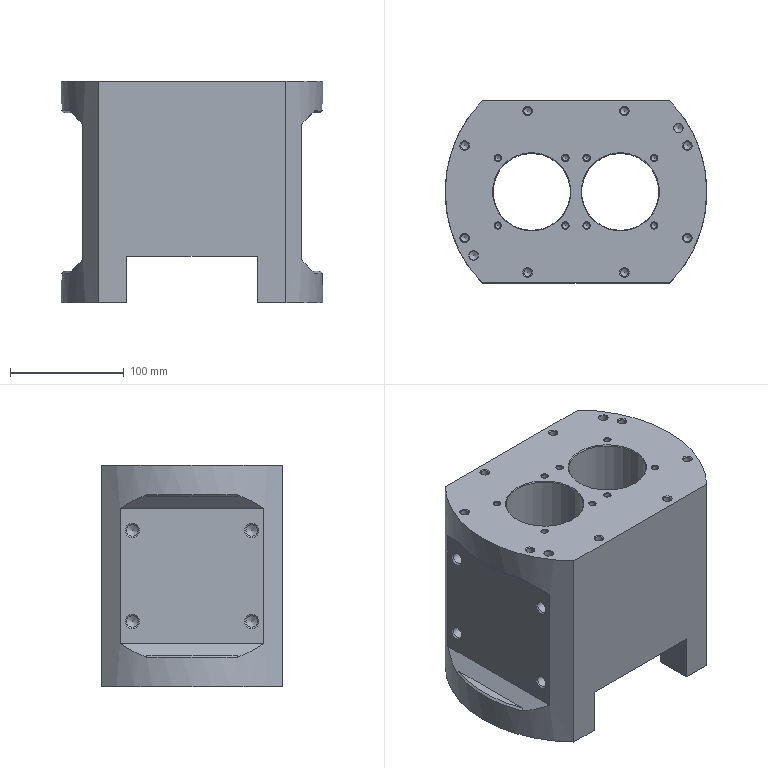NC program | NX | posted with a generic post | part box 230 x 160 x 195 mm
Lines 2897 to 3749 of 6546:
(ZLEVEL_PROFILE , TOOL : D6R0.5)
N5780 T05 M6
N5782 G54
N5784 G17 G0 G90 X68.094 Y-13.205 B0. C0. S6500 M3
N5786 G43 Z30. H5
N5788 Z2.929
N5790 G94 G1 Z-0.071 F1000.
N5792 X68.902 Y-12.621
N5794 G3 X69.147 Y-12.073 R0.6
N5796 G2 X69.147 Y12.071 R118.031 F2500.
N5798 G1 X69.145 Y12.24 Z-0.088
N5800 X69.146 Y12.409 Z-0.106
N5802 X69.147 Y12.578 Z-0.124
N5804 X69.149 Y12.747 Z-0.141
N5806 G3 X69.149 Y-12.747 R117.508
N5808 G1 X69.148 Y-12.91 Z-0.159
N5810 X69.149 Y-13.072 Z-0.177
N5812 Y-13.235 Z-0.194
N5814 X69.151 Y-13.397 Z-0.212
N5816 G2 X69.151 Y13.396 R117.429
N5818 G1 X69.149 Y13.555 Z-0.23
N5820 Y13.712 Z-0.247
N5822 Y13.87 Z-0.265
N5824 X69.153 Y14.028 Z-0.283
N5826 G3 X69.153 Y-14.028 R117.57
N5828 G1 X69.151 Y-14.174 Z-0.301
N5830 Y-14.32 Z-0.318
N5832 X69.152 Y-14.465 Z-0.336
N5834 X69.154 Y-14.611 Z-0.354
N5836 G2 X69.154 Y14.611 R117.366
N5838 G1 X69.153 Y14.757 Z-0.371
N5840 Y14.902 Z-0.389
N5842 Y15.048 Z-0.407
N5844 X69.155 Y15.193 Z-0.424
N5846 G3 X69.154 Y-15.193 R117.732
N5848 G1 X69.153 Y-15.328 Z-0.442
N5850 X69.154 Y-15.462 Z-0.46
N5852 Y-15.596 Z-0.477
N5854 X69.157 Y-15.731 Z-0.495
N5856 G2 X69.157 Y15.73 R117.468
N5858 G1 X69.156 Y15.862 Z-0.513
N5860 Y15.993 Z-0.53
N5862 Y16.125 Z-0.548
N5864 X69.157 Y16.257 Z-0.566
N5866 G3 X69.157 Y-16.256 R117.679
N5868 G1 Y-16.387 Z-0.583
N5870 Y-16.518 Z-0.601
N5872 X69.158 Y-16.649 Z-0.619
N5874 X69.16 Y-16.78 Z-0.636
N5876 G2 X69.16 Y16.782 R117.696
N5878 G1 X69.157 Y16.947 Z-0.66
N5880 X69.158 Y17.111 Z-0.684
N5882 X69.16 Y17.276 Z-0.707
N5884 G3 X69.16 Y-17.275 R117.851
N5886 G1 Y-17.434 Z-0.731
N5888 X69.161 Y-17.594 Z-0.754
N5890 X69.163 Y-17.754 Z-0.778
N5892 G2 X69.163 Y17.754 R117.723
N5894 G1 X69.162 Y17.914 Z-0.801
N5896 Y18.074 Z-0.825
N5898 X69.165 Y18.233 Z-0.849
N5900 G3 X69.164 Y-18.233 R117.882
N5902 G1 X69.162 Y-18.384 Z-0.872
N5904 X69.163 Y-18.535 Z-0.896
N5906 X69.164 Y-18.685 Z-0.919
N5908 G2 X69.164 Y18.684 R117.992
N5910 G1 X69.165 Y18.831 Z-0.943
N5912 Y18.978 Z-0.966
N5914 X69.169 Y19.124 Z-0.99
N5916 G3 X69.169 Y-19.123 R117.693
N5918 G1 X69.166 Y-19.271 Z-1.014
N5920 Y-19.417 Z-1.037
N5922 X69.171 Y-19.563 Z-1.061
N5924 G2 X69.171 Y19.564 R117.719
N5926 G1 X69.167 Y19.71 Z-1.084
N5928 Y19.856 Z-1.108
N5930 X69.171 Y20. Z-1.131
N5932 G3 X69.171 Y-19.999 R117.986
N5934 G1 X69.169 Y-20.137 Z-1.155
N5936 Y-20.274 Z-1.179
N5938 X69.17 Y-20.411 Z-1.202
N5940 G2 X69.17 Y20.411 R118.312
N5942 G1 Y20.546 Z-1.226
N5944 X69.171 Y20.682 Z-1.249
N5946 X69.174 Y20.817 Z-1.273
N5948 G3 X69.174 Y-20.818 R118.164
N5950 G1 X69.172 Y-20.953 Z-1.296
N5952 Y-21.088 Z-1.32
N5954 X69.176 Y-21.223 Z-1.344
N5956 G2 X69.177 Y21.222 R118.138
N5958 G1 X69.172 Y21.354 Z-1.367
N5960 X69.173 Y21.484 Z-1.391
N5962 X69.178 Y21.614 Z-1.414
N5964 G3 X69.178 Y-21.614 R118.128
N5966 G1 X69.175 Y-21.74 Z-1.438
N5968 Y-21.866 Z-1.461
N5970 X69.18 Y-21.992 Z-1.485
N5972 G2 X69.18 Y21.992 R118.073
N5974 G1 X69.176 Y22.119 Z-1.508
N5976 X69.177 Y22.245 Z-1.532
N5978 X69.181 Y22.37 Z-1.556
N5980 G3 X69.181 Y-22.37 R118.118
N5982 G1 X69.177 Y-22.496 Z-1.579
N5984 X69.178 Y-22.622 Z-1.603
N5986 X69.182 Y-22.748 Z-1.626
N5988 G2 X69.182 Y22.749 R118.257
N5990 G1 X69.178 Y22.873 Z-1.65
N5992 Y22.996 Z-1.673
N5994 X69.182 Y23.119 Z-1.697
N5996 G3 X69.182 Y-23.117 R118.377
N5998 G1 X69.18 Y-23.236 Z-1.721
N6000 X69.181 Y-23.355 Z-1.744
N6002 X69.183 Y-23.473 Z-1.768
N6004 G2 X69.183 Y23.474 R118.264
N6006 G1 X69.182 Y23.592 Z-1.791
N6008 Y23.71 Z-1.815
N6010 X69.185 Y23.827 Z-1.838
N6012 G3 X69.185 Y-23.826 R118.305
N6014 G1 X69.183 Y-23.945 Z-1.862
N6016 Y-24.063 Z-1.886
N6018 X69.186 Y-24.18 Z-1.909
N6020 G2 X69.186 Y24.18 R118.392
N6022 G1 X69.184 Y24.352 Z-1.945
N6024 X69.187 Y24.523 Z-1.98
N6026 G3 X69.187 Y-24.524 R118.48
N6028 G1 X69.186 Y-24.691 Z-2.015
N6030 X69.189 Y-24.856 Z-2.051
N6032 G2 X66.639 Y-4.499 R119.323
N6034 X66.693 Y5.883 R135.82
N6036 X69.189 Y24.855 R120.944
N6038 G1 X69.188 Y25.022 Z-2.086
N6040 X69.191 Y25.188 Z-2.121
N6042 G3 X66.625 Y5.883 R120.368
N6044 X66.625 Y-5.883 R181.023
N6046 X69.191 Y-25.188 R120.369
N6048 G1 X69.189 Y-25.354 Z-2.157
N6050 X69.193 Y-25.519 Z-2.192
N6052 G2 X66.596 Y-6.479 R118.044
N6054 X66.515 Y0. R174.698
N6056 X66.596 Y6.479 R174.698
N6058 X69.193 Y25.52 R118.059
N6060 G1 X69.19 Y25.687 Z-2.228
N6062 X69.194 Y25.852 Z-2.263
N6064 G3 X66.709 Y9.343 R121.287
N6066 X66.527 Y5.191 R60.135
N6068 X66.524 Y-4.845 R519.542
N6070 X66.656 Y-8.651 R67.481
N6072 X69.195 Y-25.851 R120.979
N6074 G1 X69.191 Y-26.013 Z-2.299
N6076 X69.196 Y-26.173 Z-2.334
N6078 G2 X66.596 Y-8.664 R119.128
N6080 X66.5 Y-4.088 R108.712
N6082 G1 Y4.088
N6084 G2 X66.596 Y8.664 R108.712
N6086 X69.196 Y26.174 R119.18
N6088 G1 X69.193 Y26.332 Z-2.37
N6090 X69.198 Y26.489 Z-2.405
N6092 G3 X66.596 Y9.528 R118.289
N6094 X66.5 Y5.783 R72.814
N6096 G1 Y-5.783
N6098 G3 X66.596 Y-9.528 R72.814
N6100 X69.198 Y-26.488 R118.272
N6102 G1 X69.195 Y-26.646 Z-2.441
N6104 X69.199 Y-26.801 Z-2.476
N6106 G2 X66.627 Y-10.727 R119.138
N6108 X66.5 Y-7.133 R51.
N6110 G1 Y7.133
N6112 G2 X66.627 Y10.727 R50.997
N6114 X69.199 Y26.801 R119.123
N6116 G1 X69.196 Y26.958 Z-2.512
N6118 X69.2 Y27.114 Z-2.547
N6120 G3 X66.647 Y11.766 R122.205
N6122 X66.5 Y7.478 R53.353
N6124 G1 Y-7.477
N6126 G3 X66.647 Y-11.766 R53.346
N6128 X69.2 Y-27.114 R122.268
N6130 G1 X69.197 Y-27.27 Z-2.583
N6132 X69.2 Y-27.423 Z-2.618
N6134 G2 X66.617 Y-12.112 R121.75
N6136 X66.5 Y-8.484 R50.186
N6138 G1 Y8.487
N6140 G2 X66.617 Y12.112 R50.177
N6142 X69.201 Y27.423 R121.668
N6144 G1 X69.199 Y27.573 Z-2.654
N6146 X69.201 Y27.722 Z-2.69
N6148 G3 X66.596 Y12.491 R118.29
N6150 X66.5 Y9.343 R44.651
N6152 G1 Y-9.343
N6154 G3 X66.596 Y-12.491 R44.651
N6156 X69.201 Y-27.722 R118.33
N6158 G1 X69.2 Y-27.87 Z-2.725
N6160 X69.201 Y-28.018 Z-2.761
N6162 G2 X66.835 Y-15.226 R124.638
N6164 G1 X66.775 Y-14.766
N6166 G2 X66.5 Y-10.579 R32.044
N6168 G1 Y10.579
N6170 G2 X66.775 Y14.766 R32.04
N6172 G1 X66.835 Y15.226
N6174 G2 X69.201 Y28.018 R124.597
N6176 G1 Y28.166 Z-2.796
N6178 X69.204 Y28.314 Z-2.832
N6180 G3 X66.765 Y15.247 R123.217
N6182 X66.5 Y10.963 R31.15
N6184 G1 Y-10.968
N6186 G3 X66.679 Y-14.534 R31.129
N6188 X69.204 Y-28.314 R122.319
N6190 G1 X69.203 Y-28.463 Z-2.868
N6192 X69.207 Y-28.61 Z-2.903
N6194 G2 X66.65 Y-14.88 R123.878
N6196 X66.5 Y-11.677 R32.235
N6198 G1 Y11.673
N6200 G2 X66.65 Y14.88 R32.245
N6202 X69.207 Y28.611 R123.976
N6204 G1 X69.204 Y28.76 Z-2.939
N6206 X69.209 Y28.907 Z-2.975
N6208 G3 X66.63 Y15.226 R122.218
N6210 X66.5 Y12.345 R29.755
N6212 G1 Y-12.341
N6214 G3 X66.63 Y-15.226 R29.77
N6216 X69.209 Y-28.906 R122.085
N6218 G1 X69.205 Y-29.052 Z-3.01
N6220 X69.21 Y-29.195 Z-3.046
N6222 G2 X66.613 Y-15.572 R119.558
N6224 X66.5 Y-12.975 R26.934
N6226 G1 Y12.977
N6228 G2 X66.613 Y15.572 R26.926
N6230 X69.209 Y29.196 R119.696
N6232 G1 X69.207 Y29.337 Z-3.082
N6234 X69.209 Y29.478 Z-3.118
N6236 G3 X66.68 Y16.61 R122.118
N6238 X66.5 Y13.578 R22.325
N6240 G1 Y-13.585
N6242 G3 X66.68 Y-16.61 R22.305
N6244 G1 X66.826 Y-17.648
N6246 G3 X69.239 Y-29.587 R123.791
N6248 G1 X69.223 Y-29.674 Z-3.153
N6250 X69.209 Y-29.761 Z-3.189
N6252 G2 X66.756 Y-17.648 R125.882
N6254 X66.5 Y-14.157 R21.849
N6256 G1 Y14.162
N6258 G2 X66.756 Y17.648 R21.835
N6260 X69.21 Y29.761 R125.86
N6262 G1 Y29.9 Z-3.225
N6264 X69.212 Y30.04 Z-3.261
N6266 G3 X66.76 Y18.167 R126.913
N6268 X66.5 Y14.714 R21.52
N6270 G1 Y-14.716
N6272 G3 X66.686 Y-17.648 R21.516
N6274 X69.212 Y-30.04 R125.898
N6276 G1 X69.211 Y-30.18 Z-3.296
N6278 X69.215 Y-30.319 Z-3.332
N6280 G2 X66.665 Y-17.994 R126.964
N6282 X66.5 Y-15.226 R21.69
N6284 G1 Y15.226
N6286 G2 X66.665 Y17.994 R21.69
N6288 X69.215 Y30.318 R126.807
N6290 G1 X69.212 Y30.455 Z-3.368
N6292 X69.216 Y30.59 Z-3.404
N6294 G3 X66.772 Y19.151 R128.597
N6296 X66.5 Y15.768 R20.03
N6298 G1 Y-15.766
N6300 G3 X66.654 Y-18.34 R20.036
N6302 X69.216 Y-30.592 R124.377
N6304 G1 X69.214 Y-30.726 Z-3.44
N6306 X69.216 Y-30.859 Z-3.475
N6308 G2 X66.643 Y-18.687 R122.417
N6310 X66.5 Y-16.264 R18.368
N6312 G1 Y16.264
N6314 G2 X66.754 Y19.444 R18.368
N6316 X69.216 Y30.858 R127.569
N6318 G1 X69.215 Y30.993 Z-3.511
N6320 X69.217 Y31.127 Z-3.547
N6322 G3 X66.735 Y19.697 R124.246
N6324 X66.5 Y16.756 R17.005
N6326 G1 Y-16.752
N6328 G3 X66.685 Y-19.379 R17.015
N6330 X69.217 Y-31.128 R123.32
N6332 G1 Y-31.261 Z-3.583
N6334 X69.22 Y-31.395 Z-3.619
N6336 G2 X66.73 Y-20.071 R123.281
N6338 X66.5 Y-17.228 R16.059
N6340 G1 Y17.224
N6342 G2 X66.73 Y20.071 R16.066
N6344 X69.22 Y31.395 R123.107
N6346 G1 X69.218 Y31.53 Z-3.655
N6348 X69.222 Y31.663 Z-3.691
N6350 G3 X66.775 Y20.763 R126.567
N6352 X66.5 Y17.688 R16.358
N6354 G1 Y-17.684
N6356 G3 X66.775 Y-20.763 R16.361
N6358 X69.222 Y-31.662 R126.418
N6360 G1 X69.219 Y-31.796 Z-3.726
N6362 X69.222 Y-31.928 Z-3.762
N6364 G2 X66.74 Y-20.962 R127.819
N6366 X66.5 Y-18.279 R15.107
N6368 G1 Y18.28
N6370 G2 X66.74 Y20.962 R15.095
N6372 X69.222 Y31.929 R128.024
N6374 G1 X69.22 Y32.061 Z-3.798
N6376 X69.222 Y32.192 Z-3.834
N6378 G3 X66.764 Y21.497 R131.707
N6380 X66.5 Y18.573 R15.584
N6382 G1 Y-18.57
N6384 G3 X66.696 Y-21.109 R15.59
N6386 X69.222 Y-32.192 R130.048
N6388 G1 Y-32.319 Z-3.87
N6390 X69.225 Y-32.447 Z-3.906
N6392 G2 X66.692 Y-21.454 R125.984
N6394 X66.528 Y-19.913 R10.281
N6396 G1 X66.5 Y-19.
N6398 Y18.997
N6400 G2 X66.596 Y20.837 R19.075
N6402 X67.306 Y24.569 R68.822
N6404 G1 X67.555 Y25.716
N6406 G2 X69.225 Y32.447 R119.455
N6408 G1 X69.223 Y32.575 Z-3.942
N6410 X69.227 Y32.702 Z-3.978
N6412 G3 X66.746 Y22.131 R124.885
N6414 X66.5 Y19.379 R14.123
N6416 G1 Y-19.379
N6418 G3 X66.635 Y-21.455 R14.123
N6420 X69.227 Y-32.702 R118.779
N6422 G1 X69.225 Y-32.831 Z-4.014
N6424 X69.228 Y-32.958 Z-4.05
N6426 G2 X66.685 Y-22.147 R124.585
N6428 X66.5 Y-19.826 R13.295
N6430 G1 Y19.824
N6432 G2 X66.737 Y22.436 R13.298
N6434 X69.228 Y32.958 R125.655
N6436 G1 X69.226 Y33.086 Z-4.086
N6438 X69.227 Y33.214 Z-4.122
N6440 G3 X66.681 Y22.493 R126.136
N6442 X66.5 Y20.226 R13.06
N6444 G1 Y-20.226
N6446 G3 X66.681 Y-22.493 R13.061
N6448 G1 X66.881 Y-23.531
N6450 G3 X69.227 Y-33.214 R130.713
N6452 G1 X69.226 Y-33.338 Z-4.158
N6454 X69.23 Y-33.461 Z-4.194
N6456 G2 X66.758 Y-23.271 R128.791
N6458 X66.5 Y-20.662 R13.31
N6460 G1 Y20.662
N6462 G2 X66.758 Y23.27 R13.313
N6464 X69.23 Y33.461 R128.451
N6466 G1 X69.229 Y33.584 Z-4.23
N6468 X69.232 Y33.706 Z-4.266
N6470 G3 X66.74 Y23.531 R127.446
N6472 X66.5 Y21.004 R12.742
N6474 G1 Y-21.005
N6476 G3 X66.74 Y-23.531 R12.74
N6478 X69.232 Y-33.707 R127.66
N6480 G1 X69.23 Y-33.83 Z-4.302
N6482 X69.232 Y-33.952 Z-4.339
N6484 G2 X66.756 Y-23.957 R129.272
N6486 X66.5 Y-21.444 R12.465
N6488 G1 Y21.444
N6490 G2 X66.756 Y23.958 R12.469
N6492 X69.232 Y33.951 R129.185
N6494 G1 X69.231 Y34.074 Z-4.375
N6496 X69.234 Y34.196 Z-4.411
N6498 G3 X66.785 Y24.487 R134.303
N6500 X66.5 Y21.755 R12.989
N6502 G1 Y-21.758
N6504 G3 X66.67 Y-23.877 R12.986
N6506 X69.234 Y-34.196 R128.187
N6508 G1 X69.233 Y-34.319 Z-4.447
N6510 X69.236 Y-34.44 Z-4.483
N6512 G2 X66.674 Y-24.223 R125.982
N6514 X66.5 Y-22.121 R11.961
N6516 G1 Y22.125
N6518 G2 X66.761 Y24.674 R11.955
N6520 X69.236 Y34.441 R129.306
N6522 G1 X69.234 Y34.564 Z-4.519
N6524 X69.237 Y34.686 Z-4.555
N6526 G3 X66.75 Y24.939 R128.894
N6528 X66.5 Y22.48 R11.335
N6530 G1 Y-22.483
N6532 G3 X66.678 Y-24.569 R11.33
N6534 X69.237 Y-34.685 R125.801
N6536 G1 X69.236 Y-34.808 Z-4.592
N6538 X69.237 Y-34.93 Z-4.628
N6540 G2 X66.73 Y-25.143 R127.883
N6542 X66.5 Y-22.971 R10.356
N6544 G1 Y22.973
N6546 G2 X66.73 Y25.141 R10.342
N6548 X69.237 Y34.931 R128.146
N6550 G1 X69.236 Y35.05 Z-4.664
N6552 X69.24 Y35.167 Z-4.7
N6554 G3 X66.734 Y25.482 R126.211
N6556 X66.5 Y23.299 R10.302
N6558 G1 Y-23.298
N6560 G3 X66.734 Y-25.482 R10.305
N6562 X69.24 Y-35.166 R125.977
N6564 G1 X69.238 Y-35.284 Z-4.736
N6566 X69.241 Y-35.401 Z-4.773
N6568 G2 X66.766 Y-25.954 R127.095
N6570 X66.5 Y-23.531 R10.616
N6572 G1 Y23.527
N6574 G2 X66.766 Y25.954 R10.619
N6576 X69.241 Y35.402 R127.257
N6578 G1 X69.24 Y35.519 Z-4.809
N6580 X69.241 Y35.636 Z-4.845
N6582 G3 X66.775 Y26.333 R134.359
N6584 X66.5 Y23.883 R11.067
N6586 G1 Y-23.883
N6588 G3 X66.775 Y-26.333 R11.061
N6590 X69.241 Y-35.637 R134.39
N6592 G1 Y-35.754 Z-4.881
N6594 X69.244 Y-35.871 Z-4.918
N6596 G2 X66.776 Y-26.646 R132.911
N6598 X66.5 Y-24.201 R10.582
N6600 G1 Y24.201
N6602 G2 X66.776 Y26.646 R10.585
N6604 X69.244 Y35.871 R132.704
N6606 G1 X69.243 Y35.988 Z-4.954
N6608 X69.246 Y36.104 Z-4.99
N6610 G3 X66.779 Y26.988 R135.549
N6612 X66.5 Y24.53 R10.663
N6614 G1 Y-24.532
N6616 G3 X66.705 Y-26.646 R10.661
N6618 X69.245 Y-36.105 R133.227
N6620 G1 X69.243 Y-36.222 Z-5.026
N6622 X69.245 Y-36.338 Z-5.063
N6624 G2 X66.715 Y-26.992 R135.913
N6626 X66.5 Y-24.854 R10.304
N6628 G1 Y24.859
N6630 G2 X66.775 Y27.264 R10.299
N6632 X69.245 Y36.336 R137.683
N6634 G1 X69.246 Y36.449 Z-5.099
N6636 X69.248 Y36.561 Z-5.135
N6638 G3 X66.722 Y27.308 R129.566
N6640 X66.521 Y25.792 R7.826
N6642 G1 X66.5 Y25.176
N6644 Y-25.177
N6646 X66.521 Y-25.792
N6648 G3 X66.722 Y-27.309 R7.827
N6650 X69.248 Y-36.562 R129.89
N6652 G1 X69.247 Y-36.676 Z-5.172
N6654 X69.25 Y-36.788 Z-5.208
N6656 G2 X66.666 Y-27.338 R123.437
N6658 X66.5 Y-25.494 R9.626
N6660 G1 Y25.493
N6662 G2 X66.761 Y27.784 R9.628
N6664 X69.25 Y36.787 R129.049
N6666 G1 X69.249 Y36.901 Z-5.244
N6668 X69.25 Y37.013 Z-5.281
N6670 G3 X66.756 Y28.03 R127.877
N6672 X66.5 Y25.808 R9.078
N6674 G1 Y-25.805
N6676 G3 X66.756 Y-28.03 R9.083
N6678 X69.25 Y-37.013 R127.807
N6680 G1 Y-37.126 Z-5.317
N6682 X69.253 Y-37.239 Z-5.354
N6684 G2 X66.741 Y-28.256 R124.784
N6686 X66.5 Y-26.214 R8.759
N6688 G1 Y26.214
N6690 G2 X66.741 Y28.256 R8.758
N6692 X69.253 Y37.239 R124.87
N6694 G1 X69.252 Y37.352 Z-5.39
N6696 X69.254 Y37.465 Z-5.426
N6698 G3 X66.783 Y28.722 R127.096
N6700 X66.5 Y26.42 R9.074
N6702 G1 Y-26.421
N6704 G3 X66.783 Y-28.722 R9.074
N6706 X69.255 Y-37.464 R126.814
N6708 G1 X69.254 Y-37.578 Z-5.463
N6710 X69.255 Y-37.691 Z-5.499
N6712 G2 X66.782 Y-29.019 R134.658
N6714 X66.5 Y-26.724 R9.489
N6716 G1 Y26.732
N6718 G2 X66.78 Y29.012 R9.425
N6720 X69.255 Y37.692 R135.229
N6722 G1 X69.254 Y37.803 Z-5.536
N6724 X69.257 Y37.914 Z-5.572
N6726 G3 X66.811 Y29.414 R134.223
N6728 X66.5 Y26.992 R9.175
N6730 G1 Y-26.992
N6732 G3 X66.811 Y-29.414 R9.175
N6734 X69.258 Y-37.913 R133.643
N6736 G1 X69.256 Y-38.025 Z-5.609
N6738 X69.259 Y-38.135 Z-5.645
N6740 G2 X66.74 Y-29.414 R134.868
N6742 X66.5 Y-27.316 R8.97
N6744 G1 Y27.316
N6746 G2 X66.776 Y29.562 R8.974
N6748 X69.258 Y38.136 R135.742
N6750 G1 Y38.245 Z-5.682
N6752 X69.26 Y38.354 Z-5.718
N6754 G3 X66.755 Y29.76 R140.339
N6756 X66.5 Y27.61 R8.95
N6758 G1 Y-27.607
N6760 G3 X66.755 Y-29.76 R8.952
N6762 X69.26 Y-38.353 R139.055
N6764 G1 Y-38.462 Z-5.755
N6766 X69.263 Y-38.571 Z-5.791
N6768 G2 X66.688 Y-29.76 R134.63
N6770 X66.5 Y-27.898 R9.203
N6772 G1 Y27.896
N6774 G2 X66.688 Y29.76 R9.203
N6776 X69.263 Y38.573 R135.614
N6778 G1 X69.261 Y38.683 Z-5.828
N6780 X69.263 Y38.792 Z-5.864
N6782 G3 X66.775 Y30.379 R139.759
N6784 X66.5 Y28.182 R8.441
N6786 G1 Y-28.184
N6788 G3 X66.709 Y-30.106 R8.439
N6790 X69.263 Y-38.789 R135.39
N6792 G1 Y-38.899 Z-5.901
N6794 X69.266 Y-39.008 Z-5.937
N6796 G2 X66.756 Y-30.552 R133.994
N6798 X66.5 Y-28.563 R7.867
N6800 G1 Y28.557
N6802 G2 X66.758 Y30.56 R7.91
N6804 X69.266 Y39.01 R135.299
N6806 G1 X69.264 Y39.12 Z-5.974
N6808 X69.267 Y39.228 Z-6.01
N6810 G3 X66.752 Y30.798 R135.308
N6812 X66.5 Y28.746 R7.869
N6814 G1 Y-28.747
N6816 G3 X66.752 Y-30.798 R7.868
N6818 X69.267 Y-39.225 R133.599
N6820 G1 X69.266 Y-39.333 Z-6.047
N6822 X69.267 Y-39.441 Z-6.084
N6824 G2 X66.774 Y-31.144 R136.634
N6826 X66.5 Y-29.024 R7.872
N6828 G1 Y29.023
N6830 G2 X66.774 Y31.144 R7.874
N6832 X69.265 Y39.445 R140.399
N6834 G1 Y39.554 Z-6.12
N6836 X69.268 Y39.661 Z-6.157
N6838 G3 X66.797 Y31.49 R140.895
N6840 X66.5 Y29.3 R7.938
N6842 G1 Y-29.298
N6844 G3 X66.797 Y-31.49 R7.948
N6846 X69.27 Y-39.655 R136.157
N6848 G1 X69.268 Y-39.763 Z-6.194
N6850 X69.27 Y-39.87 Z-6.23
N6852 G2 X66.792 Y-31.747 R147.325
N6854 X66.5 Y-29.578 R8.213
N6856 G1 Y29.578
N6858 G2 X66.794 Y31.757 R8.219
N6860 X69.268 Y39.879 R154.445
N6862 G1 X69.266 Y39.988 Z-6.267
N6864 X69.268 Y40.096 Z-6.304
N6866 G3 X66.807 Y32.078 R171.755
N6868 X66.5 Y29.845 R8.271
N6870 G1 Y-29.846
N6872 G3 X66.803 Y-32.06 R8.251
N6874 X69.271 Y-40.086 R157.658
N6876 G1 X69.27 Y-40.194 Z-6.34
N6878 X69.273 Y-40.301 Z-6.377
N6880 G2 X66.804 Y-32.318 R160.029
N6882 X66.5 Y-30.109 R8.172
N6884 G1 Y30.109
N6886 G2 X66.808 Y32.33 R8.176
N6888 X69.27 Y40.313 R173.185
N6890 G1 X69.264 Y40.413 Z-6.414
N6892 X69.262 Y40.511 Z-6.45
N6894 X68.923 Y39.449
N6896 X68.808 Y39.103
N6898 G3 X66.793 Y32.528 R146.839
N6900 X66.5 Y30.374 R7.916
N6902 G1 Y-30.372
N6904 G3 X66.793 Y-32.528 R7.928
N6906 X69.266 Y-40.5 R169.309
N6908 G1 X69.225 Y-40.59 Z-6.524
N6910 G2 X66.723 Y-32.528 R175.451
N6912 X66.5 Y-30.637 R8.059
N6914 G1 Y30.683
N6916 G2 X66.784 Y32.745 R7.625
N6918 X68.133 Y37.221 R124.702
N6920 G1 X69.23 Y40.63
N6922 X69.187 Y40.753 Z-6.597
N6924 X69.16 Y40.621
N6926 X68.899 Y39.795
N6928 X68.452 Y38.439
N6930 G3 X66.78 Y32.978 R135.408
N6932 X66.5 Y30.895 R7.41
N6934 G1 Y-30.895
N6936 G3 X66.752 Y-32.874 R7.41
N6938 X68.96 Y-39.987 R155.582
N6940 G2 X69.17 Y-40.687 R10.815
N6942 G1 X69.101 Y-40.787 Z-6.671
N6944 G3 X69.011 Y-40.352 R1.819
N6946 G2 X66.688 Y-32.874 R152.384
N6948 X66.5 Y-31.144 R7.743
N6950 G1 Y31.144
N6952 G2 X66.803 Y33.325 R7.743
N6954 X68.954 Y40.157 R147.413
N6956 G3 X69.108 Y40.821 R3.353
N6958 G1 X69.03 Y40.902 Z-6.744
N6960 G2 X68.922 Y40.276 R2.027
N6962 G3 X66.772 Y33.417 R145.918
N6964 X66.5 Y31.482 R7.024
N6966 G1 Y-31.483
N6968 G3 X66.772 Y-33.418 R7.01
N6970 X68.921 Y-40.284 R152.901
N6972 G2 X69.029 Y-40.903 R2.049
N6974 G1 X68.958 Y-41.036 Z-6.816
N6976 X68.915 Y-40.487
N6978 G2 X66.777 Y-33.672 R168.335
N6980 X66.5 Y-31.725 R6.977
N6982 G1 Y31.653
N6984 G2 X66.775 Y33.669 R7.11
N6986 X68.595 Y39.495 R128.973
N6988 G1 X68.647 Y39.649
N6990 X68.917 Y40.487
N6992 X68.96 Y41.033
N6994 X68.885 Y41.165 Z-6.888
N6996 X68.849 Y40.487
N6998 X68.647 Y39.849
N7000 G3 X66.779 Y33.913 R128.113
N7002 X66.5 Y31.9 R6.951
N7004 G1 Y-31.9
N7006 G3 X66.779 Y-33.913 R6.951
N7008 X68.848 Y-40.487 R169.056
N7010 G1 X68.881 Y-41.168
N7012 X68.815 Y-41.293 Z-6.959
N7014 X68.781 Y-40.487
N7016 G2 X66.812 Y-34.259 R172.094
N7018 X66.5 Y-32.144 R7.091
N7020 G1 Y32.144
N7022 G2 X66.812 Y34.259 R7.091
N7024 X68.741 Y40.326 R132.371
N7026 G3 X68.789 Y40.578 R0.89
N7028 G1 X68.819 Y41.29
N7030 X68.751 Y41.414 Z-7.031
N7032 X68.718 Y40.547
N7034 G2 X68.678 Y40.335 R0.734
N7036 G3 X66.781 Y34.384 R130.603
N7038 X66.5 Y32.424 R6.977
N7040 G1 Y-32.427
N7042 G3 X66.787 Y-34.402 R6.949
N7044 X68.714 Y-40.487 R173.207
N7046 G1 X68.746 Y-41.418
N7048 X68.673 Y-41.545 Z-7.102
N7050 X68.671 Y-41.526
N7052 X68.647 Y-40.487
N7054 G2 X66.777 Y-34.605 R185.662
N7056 X66.5 Y-32.62 R6.933
N7058 G1 Y32.62
N7060 G2 X66.777 Y34.605 R6.933
N7062 G1 X66.98 Y35.297
N7064 X68.076 Y38.757
N7066 X68.554 Y40.175
N7068 G3 X68.646 Y40.487 R4.207
N7070 G1 X68.678 Y41.539
N7072 X68.613 Y41.681 Z-7.173
N7074 X68.607 Y41.526
N7076 X68.58 Y40.563
N7078 X68.582 Y40.487
N7080 G3 X66.832 Y35.04 R328.286
N7082 X66.5 Y32.858 R7.334
N7084 G1 Y-32.86
N7086 G3 X66.821 Y-35. R7.295
N7088 X68.583 Y-40.487 R221.549
N7090 G1 X68.602 Y-41.526
N7092 X68.608 Y-41.688
N7094 X68.538 Y-41.836 Z-7.244
N7096 X68.519 Y-40.487
N7098 G2 X66.845 Y-35.297 R203.579
N7100 X66.5 Y-33.091 R7.155
N7102 G1 Y33.09
N7104 G2 X66.845 Y35.297 R7.155
N7106 X68.517 Y40.487 R208.573
N7108 G1 X68.512 Y40.578
N7110 X68.544 Y41.83
N7112 X68.508 Y41.916 Z-7.279
N7114 X68.479 Y42.001 Z-7.315
N7116 X68.472 Y41.872
N7118 X68.445 Y40.593
N7120 X68.453 Y40.487
N7122 G3 X66.815 Y35.426 R206.731
N7124 X66.5 Y33.343 R7.047
N7126 G1 Y-33.343
N7128 G3 X66.814 Y-35.422 R7.042
N7130 X68.455 Y-40.487 R195.604
N7132 G1 X68.471 Y-42.008
N7134 X68.433 Y-42.097 Z-7.35
N7136 X68.4 Y-42.187 Z-7.385
N7138 X68.399 Y-40.645
N7140 X68.391 Y-40.487
N7142 G2 X66.815 Y-35.643 R178.383
N7144 X66.5 Y-33.547 R6.86
N7146 G1 Y33.548
N7148 G2 X66.815 Y35.643 R6.862
N7150 X68.389 Y40.487 R191.2
N7152 G1 X68.38 Y40.608
N7154 X68.406 Y42.181
N7156 X68.368 Y42.271 Z-7.421
N7158 X68.337 Y42.361 Z-7.456
N7160 X68.314 Y40.834
N7162 X68.324 Y40.487
N7164 G3 X66.806 Y35.837 R169.336
N7166 X66.5 Y33.776 R6.804
N7168 G1 Y-33.775
N7170 G3 X66.749 Y-35.643 R6.804
N7172 G1 X66.858 Y-35.989
N7174 G3 X68.327 Y-40.487 R148.706
N7176 G1 X68.334 Y-40.66
N7178 X68.333 Y-42.365
N7180 X68.295 Y-42.455 Z-7.491
N7182 X68.261 Y-42.544 Z-7.527
N7184 Y-40.487
N7186 G2 X66.791 Y-35.989 R143.242
N7188 X66.5 Y-34.002 R6.471
N7190 G1 Y34.
N7192 G2 X66.791 Y35.989 R6.474
N7194 X68.26 Y40.487 R150.553
N7196 G1 X68.248 Y40.834
N7198 X68.264 Y42.541
N7200 X68.229 Y42.631 Z-7.562
N7202 X68.198 Y42.72 Z-7.597
N7204 X68.193 Y42.564
N7206 X68.184 Y40.834
N7208 X68.195 Y40.697
N7210 Y40.487
N7212 G3 X66.797 Y36.234 R127.575
N7214 X66.5 Y34.223 R6.659
N7216 G1 Y-34.223
N7218 G3 X66.727 Y-35.989 R6.661
N7220 X68.195 Y-40.487 R136.851
N7222 G1 X68.191 Y-42.564
N7224 X68.196 Y-42.723
N7226 X68.158 Y-42.812 Z-7.633
N7228 X68.123 Y-42.902 Z-7.668
N7230 X68.121 Y-42.564
N7232 X68.123 Y-40.909
N7234 X68.125 Y-40.877
N7236 Y-40.483
N7238 G2 X66.768 Y-36.335 R144.174
N7240 X66.5 Y-34.445 R6.36
N7242 G1 Y34.446
N7244 G2 X66.768 Y36.335 R6.36
N7246 X68.125 Y40.483 R144.174
N7248 G1 Y40.872
N7250 X68.118 Y40.917
N7252 X68.124 Y42.9
N7254 X68.089 Y42.988 Z-7.703
N7256 X68.058 Y43.075 Z-7.739
N7258 X68.053 Y42.91
N7260 X68.05 Y41.18
N7262 X68.054 Y40.834
N7264 Y40.47
N7266 G3 X66.811 Y36.681 R135.378
N7268 X66.5 Y34.668 R6.394
N7270 G1 Y-34.667
N7272 G3 X66.811 Y-36.681 R6.395
N7274 X68.054 Y-40.47 R137.079
N7276 G1 Y-41.091
N7278 X68.053 Y-42.91
N7280 X68.057 Y-43.076
N7282 X68.017 Y-43.164 Z-7.774
N7284 X67.982 Y-43.251 Z-7.81
N7286 X67.983 Y-41.277
N7288 Y-40.457
N7290 G2 X66.792 Y-36.832 R134.498
N7292 X66.5 Y-34.925 R6.385
N7294 G1 Y34.925
N7296 G2 X66.792 Y36.832 R6.385
N7298 X67.983 Y40.457 R134.411
N7300 G1 Y41.277
N7302 Y43.25
N7304 X67.948 Y43.337 Z-7.845
N7306 X67.915 Y43.425 Z-7.88
N7308 X67.913 Y41.46
N7310 Y40.444
N7312 G3 X66.787 Y37.027 R129.807
N7314 X66.5 Y35.102 R6.298
N7316 G1 Y-35.102
N7318 G3 X66.787 Y-37.027 R6.298
N7320 X67.913 Y-40.444 R129.807
N7322 G1 Y-41.46
N7324 X67.912 Y-41.526
N7326 Y-43.256
N7328 X67.915 Y-43.425
N7330 X67.876 Y-43.513 Z-7.916
N7332 X67.841 Y-43.6 Z-7.951
N7334 Y-41.644
N7336 X67.842 Y-41.526
N7338 Y-40.431
N7340 G2 X66.793 Y-37.252 R116.909
N7342 X66.5 Y-35.343 R6.37
N7344 G1 Y35.343
N7346 G2 X66.793 Y37.252 R6.371
N7348 X67.842 Y40.431 R116.909
N7350 G1 Y41.526
N7352 X67.839 Y41.872
N7354 X67.842 Y43.599
N7356 X67.806 Y43.687 Z-7.986
N7358 X67.777 Y43.774 Z-8.022
N7360 X67.771 Y43.602
N7362 X67.769 Y41.872
N7364 X67.771 Y41.526
N7366 Y40.418
N7368 G3 X66.799 Y37.486 R123.867
N7370 X66.5 Y35.558 R6.363
N7372 G1 Y-35.558
N7374 G3 X66.799 Y-37.486 R6.363
N7376 X67.771 Y-40.418 R123.867
N7378 G1 Y-41.526
N7380 X67.77 Y-41.825
N7382 X67.771 Y-43.602
N7384 X67.777 Y-43.774
N7386 X67.735 Y-43.861 Z-8.057
N7388 X67.7 Y-43.949 Z-8.092
N7390 X67.699 Y-42.007
N7392 X67.701 Y-41.872
N7394 Y-40.405
N7396 X66.916 Y-38.065
N7398 X66.806 Y-37.719
N7400 G2 X66.5 Y-35.747 R6.353
N7402 G1 Y35.746
N7404 G2 X66.806 Y37.719 R6.354
N7406 G1 X66.916 Y38.065
N7408 X67.701 Y40.405
N7410 Y41.872
N7412 X67.699 Y42.007
N7414 X67.7 Y43.949
N7416 X67.665 Y44.036 Z-8.128
N7418 X67.632 Y44.123 Z-8.163
N7420 X67.63 Y43.948
N7422 Y41.872
N7424 X67.629 Y40.382
N7426 X66.96 Y38.411
N7428 X66.809 Y37.94
N7430 G3 X66.5 Y35.972 R6.429
N7432 G1 Y-35.972
N7434 G3 X66.809 Y-37.94 R6.429
N7436 G1 X66.96 Y-38.411
N7438 X67.629 Y-40.382
N7440 X67.63 Y-42.185
N7442 Y-43.948
N7444 X67.632 Y-44.123
N7446 X67.594 Y-44.21 Z-8.198
N7448 X67.559 Y-44.298 Z-8.234
N7450 Y-42.363
N7452 X67.558 Y-40.369
N7454 X66.844 Y-38.265
N7456 G2 X66.5 Y-36.183 R6.476
N7458 G1 Y36.183
N7460 G2 X66.844 Y38.265 R6.476
N7462 G1 X67.558 Y40.369
N7464 X67.559 Y42.363
N7466 Y44.298
N7468 X67.524 Y44.382 Z-8.269
N7470 X67.493 Y44.466 Z-8.305
N7472 X67.488 Y44.294
N7474 Y42.541
N7476 Y40.356
N7478 X66.827 Y38.411